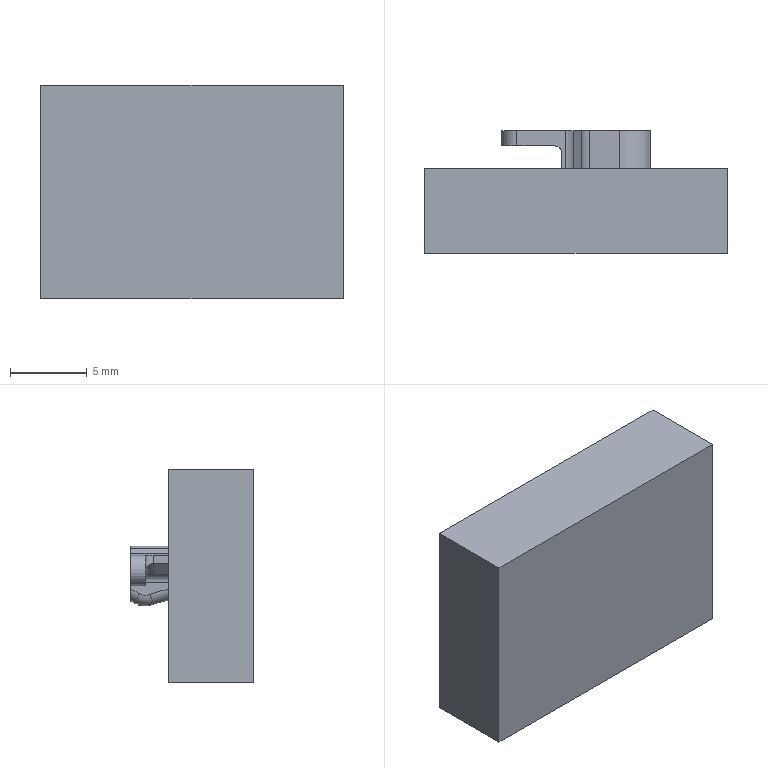NC program | NX | posted with a generic post | part box 19.7 x 8 x 13.91 mm
Lines 1 to 44 of 12778:
N10 G17 G21 G94 G90
(FLOOR_WALL , TOOL : D10JING)
N12 T10 M6
N14 G54
N16 G17 G0 G90 X-14.85 Y5.452 B0. C0. S5000 M3
N18 G43 Z30. H10
N20 Z3.
N22 G94 G1 Z0. F1250.
N24 X-11.85
N26 X11.85
N28 Y1.999
N30 X-11.85
N32 Y-1.455
N34 X11.85
N36 X14.85
N38 Z3.
N40 G0 Z30.
N42 M5
(DRILLING , TOOL : ZXZ)
N44 T01 M6
N46 G54
N48 G17 G0 G90 X3.85 Y-0.355 B0. C0. S5000 M3
N50 G43 Z30. H1
N52 G94 G81 G98 Z-0.6 F250. R3.
N54 G80
N56 G0 X3.85 Y-0.355 Z30.
N58 M5
(DRILLING_COPY , TOOL : 1.0ZT)
N60 T11 M6
N62 G54
N64 G17 G0 G90 X3.85 Y-0.355 B0. C0. S2000 M3
N66 G43 Z30. H11
N68 G94 G83 G98 Z-7.3 F100. Q0.5 R3.
N70 G80
N72 G0 X3.85 Y-0.355 Z30.
N74 M5